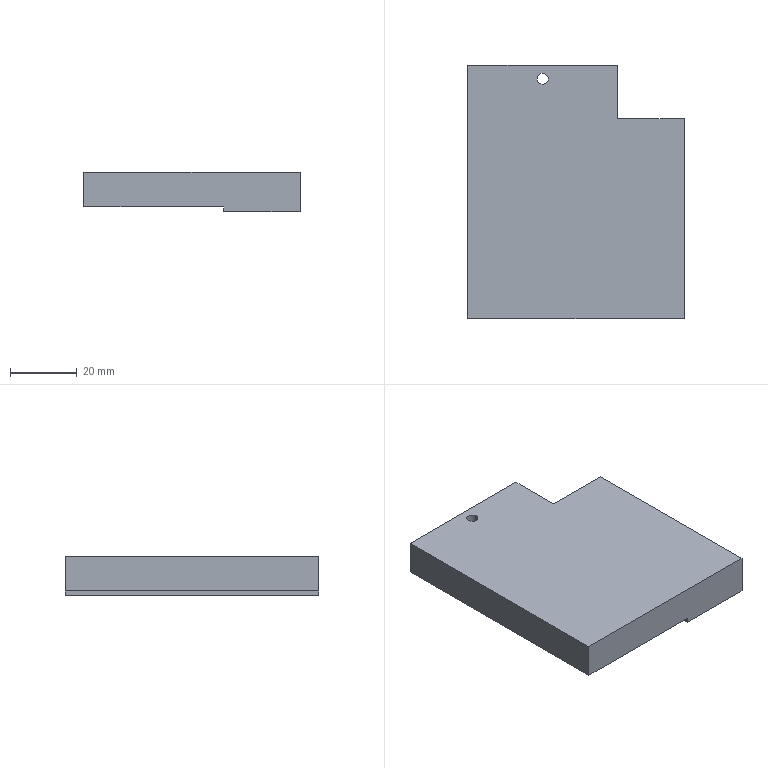Part | SolidWorks | features ICE 2, 3DProfileFeature 1, Extrusion 1, HoleWzd 1 | 1 solid | 12 faces | box 65 x 76 x 12 mm | volume 50562 mm3 | plane 10 | cylinder 2 | commonest cylinder face diameters 3.3 x2
STEP:
#1=CARTESIAN_POINT('',(-11.65,42.,1.5));
#2=VERTEX_POINT('',#1);
#3=CARTESIAN_POINT('',(-8.35,42.,1.5));
#4=VERTEX_POINT('',#3);
#5=CARTESIAN_POINT('',(-10.,42.,1.5));
#6=DIRECTION('',(0.,0.,1.));
#7=DIRECTION('',(1.,0.,0.));
#8=AXIS2_PLACEMENT_3D('',#5,#6,#7);
#9=CIRCLE('',#8,1.65);
#10=EDGE_CURVE('',#2,#4,#9,.T.);
#11=ORIENTED_EDGE('',*,*,#10,.F.);
#12=CARTESIAN_POINT('',(-11.65,42.,12.));
#13=VERTEX_POINT('',#12);
#14=CARTESIAN_POINT('',(-11.65,42.,12.));
#15=DIRECTION('',(0.,0.,1.));
#16=VECTOR('',#15,1000.);
#17=LINE('',#14,#16);
#18=EDGE_CURVE('',#2,#13,#17,.T.);
#19=ORIENTED_EDGE('',*,*,#18,.T.);
#20=CARTESIAN_POINT('',(-8.35,42.,12.));
#21=VERTEX_POINT('',#20);
#22=CARTESIAN_POINT('',(-10.,42.,12.));
#23=DIRECTION('',(0.,0.,1.));
#24=DIRECTION('',(1.,0.,0.));
#25=AXIS2_PLACEMENT_3D('',#22,#23,#24);
#26=CIRCLE('',#25,1.65);
#27=EDGE_CURVE('',#13,#21,#26,.T.);
#28=ORIENTED_EDGE('',*,*,#27,.T.);
#29=CARTESIAN_POINT('',(-8.35,42.,12.));
#30=DIRECTION('',(0.,0.,1.));
#31=VECTOR('',#30,1000.);
#32=LINE('',#29,#31);
#33=EDGE_CURVE('',#4,#21,#32,.T.);
#34=ORIENTED_EDGE('',*,*,#33,.F.);
#35=EDGE_LOOP('',(#11,#19,#28,#34));
#36=FACE_OUTER_BOUND('',#35,.T.);
#37=CARTESIAN_POINT('',(-10.,42.,12.));
#38=DIRECTION('',(0.,0.,1.));
#39=DIRECTION('',(1.,0.,0.));
#40=AXIS2_PLACEMENT_3D('',#37,#38,#39);
#41=CYLINDRICAL_SURFACE('',#40,1.65);
#42=ADVANCED_FACE('',(#36),#41,.F.);
#43=CARTESIAN_POINT('',(12.5,30.,12.));
#44=VERTEX_POINT('',#43);
#45=CARTESIAN_POINT('',(12.5,30.,0.));
#46=VERTEX_POINT('',#45);
#47=CARTESIAN_POINT('',(12.5,30.,59.76));
#48=DIRECTION('',(0.,0.,-1.));
#49=VECTOR('',#48,1000.);
#50=LINE('',#47,#49);
#51=EDGE_CURVE('',#44,#46,#50,.T.);
#52=ORIENTED_EDGE('',*,*,#51,.F.);
#53=CARTESIAN_POINT('',(32.5,30.,12.));
#54=VERTEX_POINT('',#53);
#55=CARTESIAN_POINT('',(-32.5,30.,12.));
#56=DIRECTION('',(-1.,0.,0.));
#57=VECTOR('',#56,1000.);
#58=LINE('',#55,#57);
#59=EDGE_CURVE('',#54,#44,#58,.T.);
#60=ORIENTED_EDGE('',*,*,#59,.F.);
#61=CARTESIAN_POINT('',(32.5,30.,0.));
#62=VERTEX_POINT('',#61);
#63=CARTESIAN_POINT('',(32.5,30.,12.));
#64=DIRECTION('',(0.,0.,-1.));
#65=VECTOR('',#64,1000.);
#66=LINE('',#63,#65);
#67=EDGE_CURVE('',#54,#62,#66,.T.);
#68=ORIENTED_EDGE('',*,*,#67,.T.);
#69=CARTESIAN_POINT('',(-32.5,30.,0.));
#70=DIRECTION('',(-1.,0.,0.));
#71=VECTOR('',#70,1000.);
#72=LINE('',#69,#71);
#73=EDGE_CURVE('',#62,#46,#72,.T.);
#74=ORIENTED_EDGE('',*,*,#73,.T.);
#75=EDGE_LOOP('',(#52,#60,#68,#74));
#76=FACE_OUTER_BOUND('',#75,.T.);
#77=CARTESIAN_POINT('',(-32.5,30.,12.));
#78=DIRECTION('',(0.,-1.,0.));
#79=DIRECTION('',(0.,0.,-1.));
#80=AXIS2_PLACEMENT_3D('',#77,#78,#79);
#81=PLANE('',#80);
#82=ADVANCED_FACE('',(#76),#81,.F.);
#83=CARTESIAN_POINT('',(32.5,-30.,0.));
#84=VERTEX_POINT('',#83);
#85=CARTESIAN_POINT('',(32.5,-30.,0.));
#86=DIRECTION('',(0.,1.,0.));
#87=VECTOR('',#86,1000.);
#88=LINE('',#85,#87);
#89=EDGE_CURVE('',#84,#62,#88,.T.);
#90=ORIENTED_EDGE('',*,*,#89,.T.);
#91=ORIENTED_EDGE('',*,*,#67,.F.);
#92=CARTESIAN_POINT('',(32.5,-30.,12.));
#93=VERTEX_POINT('',#92);
#94=CARTESIAN_POINT('',(32.5,-30.,12.));
#95=DIRECTION('',(0.,1.,0.));
#96=VECTOR('',#95,1000.);
#97=LINE('',#94,#96);
#98=EDGE_CURVE('',#93,#54,#97,.T.);
#99=ORIENTED_EDGE('',*,*,#98,.F.);
#100=CARTESIAN_POINT('',(32.5,-30.,12.));
#101=DIRECTION('',(0.,0.,-1.));
#102=VECTOR('',#101,1000.);
#103=LINE('',#100,#102);
#104=EDGE_CURVE('',#93,#84,#103,.T.);
#105=ORIENTED_EDGE('',*,*,#104,.T.);
#106=EDGE_LOOP('',(#90,#91,#99,#105));
#107=FACE_OUTER_BOUND('',#106,.T.);
#108=CARTESIAN_POINT('',(32.5,-30.,12.));
#109=DIRECTION('',(-1.,0.,0.));
#110=DIRECTION('',(0.,0.,1.));
#111=AXIS2_PLACEMENT_3D('',#108,#109,#110);
#112=PLANE('',#111);
#113=ADVANCED_FACE('',(#107),#112,.F.);
#114=CARTESIAN_POINT('',(-32.5,46.,12.));
#115=VERTEX_POINT('',#114);
#116=CARTESIAN_POINT('',(-32.5,46.,1.5));
#117=VERTEX_POINT('',#116);
#118=CARTESIAN_POINT('',(-32.5,46.,59.76));
#119=DIRECTION('',(0.,0.,-1.));
#120=VECTOR('',#119,1000.);
#121=LINE('',#118,#120);
#122=EDGE_CURVE('',#115,#117,#121,.T.);
#123=ORIENTED_EDGE('',*,*,#122,.T.);
#124=CARTESIAN_POINT('',(-32.5,-30.,1.5));
#125=VERTEX_POINT('',#124);
#126=CARTESIAN_POINT('',(-32.5,46.,1.5));
#127=DIRECTION('',(0.,1.,0.));
#128=VECTOR('',#127,1000.);
#129=LINE('',#126,#128);
#130=EDGE_CURVE('',#125,#117,#129,.T.);
#131=ORIENTED_EDGE('',*,*,#130,.F.);
#132=CARTESIAN_POINT('',(-32.5,-30.,12.));
#133=VERTEX_POINT('',#132);
#134=CARTESIAN_POINT('',(-32.5,-30.,12.));
#135=DIRECTION('',(0.,0.,-1.));
#136=VECTOR('',#135,1000.);
#137=LINE('',#134,#136);
#138=EDGE_CURVE('',#133,#125,#137,.T.);
#139=ORIENTED_EDGE('',*,*,#138,.F.);
#140=CARTESIAN_POINT('',(-32.5,-30.,12.));
#141=DIRECTION('',(0.,-1.,0.));
#142=VECTOR('',#141,1000.);
#143=LINE('',#140,#142);
#144=EDGE_CURVE('',#115,#133,#143,.T.);
#145=ORIENTED_EDGE('',*,*,#144,.F.);
#146=EDGE_LOOP('',(#123,#131,#139,#145));
#147=FACE_OUTER_BOUND('',#146,.T.);
#148=CARTESIAN_POINT('',(-32.5,-30.,12.));
#149=DIRECTION('',(1.,0.,0.));
#150=DIRECTION('',(0.,0.,-1.));
#151=AXIS2_PLACEMENT_3D('',#148,#149,#150);
#152=PLANE('',#151);
#153=ADVANCED_FACE('',(#147),#152,.F.);
#154=CARTESIAN_POINT('',(9.5,-30.,1.5));
#155=VERTEX_POINT('',#154);
#156=CARTESIAN_POINT('',(-32.5,-30.,1.5));
#157=DIRECTION('',(-1.,0.,0.));
#158=VECTOR('',#157,1000.);
#159=LINE('',#156,#158);
#160=EDGE_CURVE('',#155,#125,#159,.T.);
#161=ORIENTED_EDGE('',*,*,#160,.F.);
#162=CARTESIAN_POINT('',(9.5,-30.,0.));
#163=VERTEX_POINT('',#162);
#164=CARTESIAN_POINT('',(9.5,-30.,1.5));
#165=DIRECTION('',(0.,0.,-1.));
#166=VECTOR('',#165,1000.);
#167=LINE('',#164,#166);
#168=EDGE_CURVE('',#155,#163,#167,.T.);
#169=ORIENTED_EDGE('',*,*,#168,.T.);
#170=CARTESIAN_POINT('',(-32.5,-30.,0.));
#171=DIRECTION('',(1.,0.,0.));
#172=VECTOR('',#171,1000.);
#173=LINE('',#170,#172);
#174=EDGE_CURVE('',#163,#84,#173,.T.);
#175=ORIENTED_EDGE('',*,*,#174,.T.);
#176=ORIENTED_EDGE('',*,*,#104,.F.);
#177=CARTESIAN_POINT('',(-32.5,-30.,12.));
#178=DIRECTION('',(1.,0.,0.));
#179=VECTOR('',#178,1000.);
#180=LINE('',#177,#179);
#181=EDGE_CURVE('',#133,#93,#180,.T.);
#182=ORIENTED_EDGE('',*,*,#181,.F.);
#183=ORIENTED_EDGE('',*,*,#138,.T.);
#184=EDGE_LOOP('',(#161,#169,#175,#176,#182,#183));
#185=FACE_OUTER_BOUND('',#184,.T.);
#186=CARTESIAN_POINT('',(-32.5,-30.,12.));
#187=DIRECTION('',(0.,1.,0.));
#188=DIRECTION('',(0.,0.,1.));
#189=AXIS2_PLACEMENT_3D('',#186,#187,#188);
#190=PLANE('',#189);
#191=ADVANCED_FACE('',(#185),#190,.F.);
#192=CARTESIAN_POINT('',(-10.,42.,12.));
#193=DIRECTION('',(0.,0.,1.));
#194=DIRECTION('',(1.,0.,0.));
#195=AXIS2_PLACEMENT_3D('',#192,#193,#194);
#196=CIRCLE('',#195,1.65);
#197=EDGE_CURVE('',#21,#13,#196,.T.);
#198=ORIENTED_EDGE('',*,*,#197,.F.);
#199=ORIENTED_EDGE('',*,*,#27,.F.);
#200=EDGE_LOOP('',(#198,#199));
#201=FACE_BOUND('',#200,.T.);
#202=ORIENTED_EDGE('',*,*,#98,.T.);
#203=ORIENTED_EDGE('',*,*,#59,.T.);
#204=CARTESIAN_POINT('',(12.5,46.,12.));
#205=VERTEX_POINT('',#204);
#206=CARTESIAN_POINT('',(12.5,30.,12.));
#207=DIRECTION('',(0.,1.,0.));
#208=VECTOR('',#207,1000.);
#209=LINE('',#206,#208);
#210=EDGE_CURVE('',#44,#205,#209,.T.);
#211=ORIENTED_EDGE('',*,*,#210,.T.);
#212=CARTESIAN_POINT('',(12.5,46.,12.));
#213=DIRECTION('',(-1.,0.,0.));
#214=VECTOR('',#213,1000.);
#215=LINE('',#212,#214);
#216=EDGE_CURVE('',#205,#115,#215,.T.);
#217=ORIENTED_EDGE('',*,*,#216,.T.);
#218=ORIENTED_EDGE('',*,*,#144,.T.);
#219=ORIENTED_EDGE('',*,*,#181,.T.);
#220=EDGE_LOOP('',(#202,#203,#211,#217,#218,#219));
#221=FACE_OUTER_BOUND('',#220,.T.);
#222=CARTESIAN_POINT('',(0.,0.,12.));
#223=DIRECTION('',(0.,0.,-1.));
#224=DIRECTION('',(-1.,0.,0.));
#225=AXIS2_PLACEMENT_3D('',#222,#223,#224);
#226=PLANE('',#225);
#227=ADVANCED_FACE('',(#201,#221),#226,.F.);
#228=CARTESIAN_POINT('',(9.5,46.,0.));
#229=VERTEX_POINT('',#228);
#230=CARTESIAN_POINT('',(9.5,46.,0.));
#231=DIRECTION('',(0.,-1.,0.));
#232=VECTOR('',#231,1000.);
#233=LINE('',#230,#232);
#234=EDGE_CURVE('',#229,#163,#233,.T.);
#235=ORIENTED_EDGE('',*,*,#234,.F.);
#236=CARTESIAN_POINT('',(12.5,46.,0.));
#237=VERTEX_POINT('',#236);
#238=CARTESIAN_POINT('',(12.5,46.,0.));
#239=DIRECTION('',(1.,0.,0.));
#240=VECTOR('',#239,1000.);
#241=LINE('',#238,#240);
#242=EDGE_CURVE('',#229,#237,#241,.T.);
#243=ORIENTED_EDGE('',*,*,#242,.T.);
#244=CARTESIAN_POINT('',(12.5,30.,0.));
#245=DIRECTION('',(0.,-1.,0.));
#246=VECTOR('',#245,1000.);
#247=LINE('',#244,#246);
#248=EDGE_CURVE('',#237,#46,#247,.T.);
#249=ORIENTED_EDGE('',*,*,#248,.T.);
#250=ORIENTED_EDGE('',*,*,#73,.F.);
#251=ORIENTED_EDGE('',*,*,#89,.F.);
#252=ORIENTED_EDGE('',*,*,#174,.F.);
#253=EDGE_LOOP('',(#235,#243,#249,#250,#251,#252));
#254=FACE_OUTER_BOUND('',#253,.T.);
#255=CARTESIAN_POINT('',(0.,0.,0.));
#256=DIRECTION('',(0.,0.,-1.));
#257=DIRECTION('',(-1.,0.,0.));
#258=AXIS2_PLACEMENT_3D('',#255,#256,#257);
#259=PLANE('',#258);
#260=ADVANCED_FACE('',(#254),#259,.T.);
#261=ORIENTED_EDGE('',*,*,#210,.F.);
#262=ORIENTED_EDGE('',*,*,#51,.T.);
#263=ORIENTED_EDGE('',*,*,#248,.F.);
#264=CARTESIAN_POINT('',(12.5,46.,59.76));
#265=DIRECTION('',(0.,0.,-1.));
#266=VECTOR('',#265,1000.);
#267=LINE('',#264,#266);
#268=EDGE_CURVE('',#205,#237,#267,.T.);
#269=ORIENTED_EDGE('',*,*,#268,.F.);
#270=EDGE_LOOP('',(#261,#262,#263,#269));
#271=FACE_OUTER_BOUND('',#270,.T.);
#272=CARTESIAN_POINT('',(12.5,30.,59.76));
#273=DIRECTION('',(1.,0.,0.));
#274=DIRECTION('',(0.,0.,-1.));
#275=AXIS2_PLACEMENT_3D('',#272,#273,#274);
#276=PLANE('',#275);
#277=ADVANCED_FACE('',(#271),#276,.T.);
#278=CARTESIAN_POINT('',(9.5,46.,1.5));
#279=VERTEX_POINT('',#278);
#280=CARTESIAN_POINT('',(9.5,46.,1.5));
#281=DIRECTION('',(0.,0.,-1.));
#282=VECTOR('',#281,1000.);
#283=LINE('',#280,#282);
#284=EDGE_CURVE('',#279,#229,#283,.T.);
#285=ORIENTED_EDGE('',*,*,#284,.F.);
#286=CARTESIAN_POINT('',(-32.5,46.,1.5));
#287=DIRECTION('',(1.,0.,0.));
#288=VECTOR('',#287,1000.);
#289=LINE('',#286,#288);
#290=EDGE_CURVE('',#117,#279,#289,.T.);
#291=ORIENTED_EDGE('',*,*,#290,.F.);
#292=ORIENTED_EDGE('',*,*,#122,.F.);
#293=ORIENTED_EDGE('',*,*,#216,.F.);
#294=ORIENTED_EDGE('',*,*,#268,.T.);
#295=ORIENTED_EDGE('',*,*,#242,.F.);
#296=EDGE_LOOP('',(#285,#291,#292,#293,#294,#295));
#297=FACE_OUTER_BOUND('',#296,.T.);
#298=CARTESIAN_POINT('',(12.5,46.,59.76));
#299=DIRECTION('',(0.,1.,0.));
#300=DIRECTION('',(0.,0.,1.));
#301=AXIS2_PLACEMENT_3D('',#298,#299,#300);
#302=PLANE('',#301);
#303=ADVANCED_FACE('',(#297),#302,.T.);
#304=ORIENTED_EDGE('',*,*,#234,.T.);
#305=ORIENTED_EDGE('',*,*,#168,.F.);
#306=CARTESIAN_POINT('',(9.5,46.,1.5));
#307=DIRECTION('',(0.,-1.,0.));
#308=VECTOR('',#307,1000.);
#309=LINE('',#306,#308);
#310=EDGE_CURVE('',#279,#155,#309,.T.);
#311=ORIENTED_EDGE('',*,*,#310,.F.);
#312=ORIENTED_EDGE('',*,*,#284,.T.);
#313=EDGE_LOOP('',(#304,#305,#311,#312));
#314=FACE_OUTER_BOUND('',#313,.T.);
#315=CARTESIAN_POINT('',(9.5,46.,1.5));
#316=DIRECTION('',(1.,0.,0.));
#317=DIRECTION('',(0.,1.,0.));
#318=AXIS2_PLACEMENT_3D('',#315,#316,#317);
#319=PLANE('',#318);
#320=ADVANCED_FACE('',(#314),#319,.F.);
#321=CARTESIAN_POINT('',(-10.,42.,1.5));
#322=DIRECTION('',(0.,0.,1.));
#323=DIRECTION('',(1.,0.,0.));
#324=AXIS2_PLACEMENT_3D('',#321,#322,#323);
#325=CIRCLE('',#324,1.65);
#326=EDGE_CURVE('',#4,#2,#325,.T.);
#327=ORIENTED_EDGE('',*,*,#326,.T.);
#328=ORIENTED_EDGE('',*,*,#10,.T.);
#329=EDGE_LOOP('',(#327,#328));
#330=FACE_BOUND('',#329,.T.);
#331=ORIENTED_EDGE('',*,*,#130,.T.);
#332=ORIENTED_EDGE('',*,*,#290,.T.);
#333=ORIENTED_EDGE('',*,*,#310,.T.);
#334=ORIENTED_EDGE('',*,*,#160,.T.);
#335=EDGE_LOOP('',(#331,#332,#333,#334));
#336=FACE_OUTER_BOUND('',#335,.T.);
#337=CARTESIAN_POINT('',(0.,0.,1.5));
#338=DIRECTION('',(0.,0.,1.));
#339=DIRECTION('',(1.,0.,0.));
#340=AXIS2_PLACEMENT_3D('',#337,#338,#339);
#341=PLANE('',#340);
#342=ADVANCED_FACE('',(#330,#336),#341,.F.);
#343=ORIENTED_EDGE('',*,*,#18,.F.);
#344=ORIENTED_EDGE('',*,*,#326,.F.);
#345=ORIENTED_EDGE('',*,*,#33,.T.);
#346=ORIENTED_EDGE('',*,*,#197,.T.);
#347=EDGE_LOOP('',(#343,#344,#345,#346));
#348=FACE_OUTER_BOUND('',#347,.T.);
#349=CARTESIAN_POINT('',(-10.,42.,12.));
#350=DIRECTION('',(0.,0.,1.));
#351=DIRECTION('',(1.,0.,0.));
#352=AXIS2_PLACEMENT_3D('',#349,#350,#351);
#353=CYLINDRICAL_SURFACE('',#352,1.65);
#354=ADVANCED_FACE('',(#348),#353,.F.);
#355=CLOSED_SHELL('',(#42,#82,#113,#153,#191,#227,#260,#277,#303,#320,#342,#354));
#356=MANIFOLD_SOLID_BREP('',#355);
#357=CARTESIAN_POINT('',(0.,0.,0.));
#358=DIRECTION('',(0.,0.,1.));
#359=DIRECTION('',(1.,0.,0.));
#360=AXIS2_PLACEMENT_3D('',#357,#358,#359);
#361=(LENGTH_UNIT()NAMED_UNIT(*)SI_UNIT(.MILLI.,.METRE.));
#362=UNCERTAINTY_MEASURE_WITH_UNIT(LENGTH_MEASURE(0.00001),#361,'','');
#363=(NAMED_UNIT(*)PLANE_ANGLE_UNIT()SI_UNIT($,.RADIAN.));
#364=(NAMED_UNIT(*)SI_UNIT($,.STERADIAN.)SOLID_ANGLE_UNIT());
#365=(GEOMETRIC_REPRESENTATION_CONTEXT(3)GLOBAL_UNCERTAINTY_ASSIGNED_CONTEXT((#362))GLOBAL_UNIT_ASSIGNED_CONTEXT((#361,#363,#364))REPRESENTATION_CONTEXT('',''));
#366=ADVANCED_BREP_SHAPE_REPRESENTATION('',(#356,#360),#365);